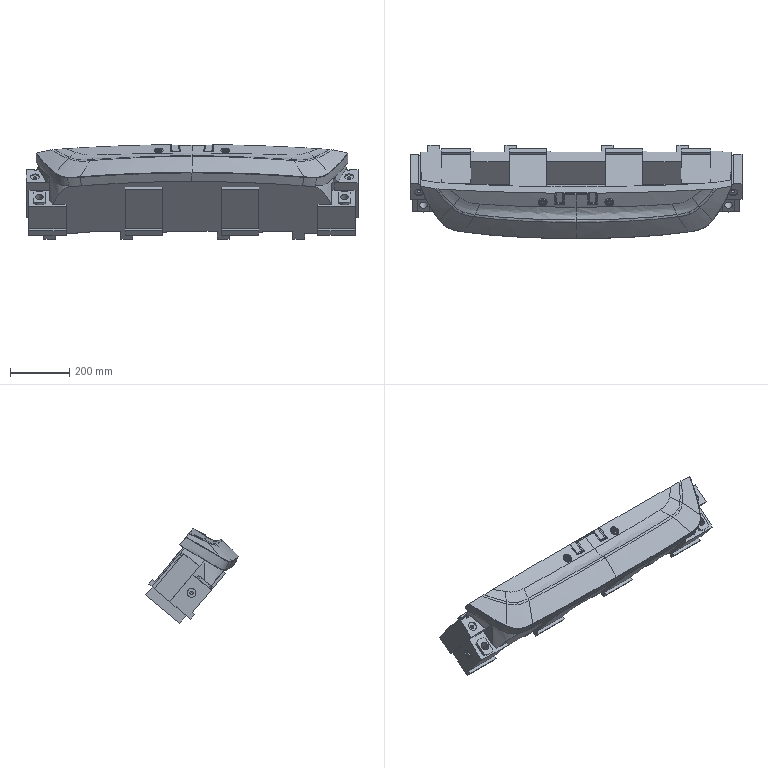Part | NX | features solid 2 | 1 solid | 271 faces | box 1120 x 314.485 x 319.837 mm | volume 35843661 mm3 | plane 135 | spline 118 | cylinder 14 | cone 4 | commonest cylinder face diameters 12 x4 30 x4 60 x4 27 x2